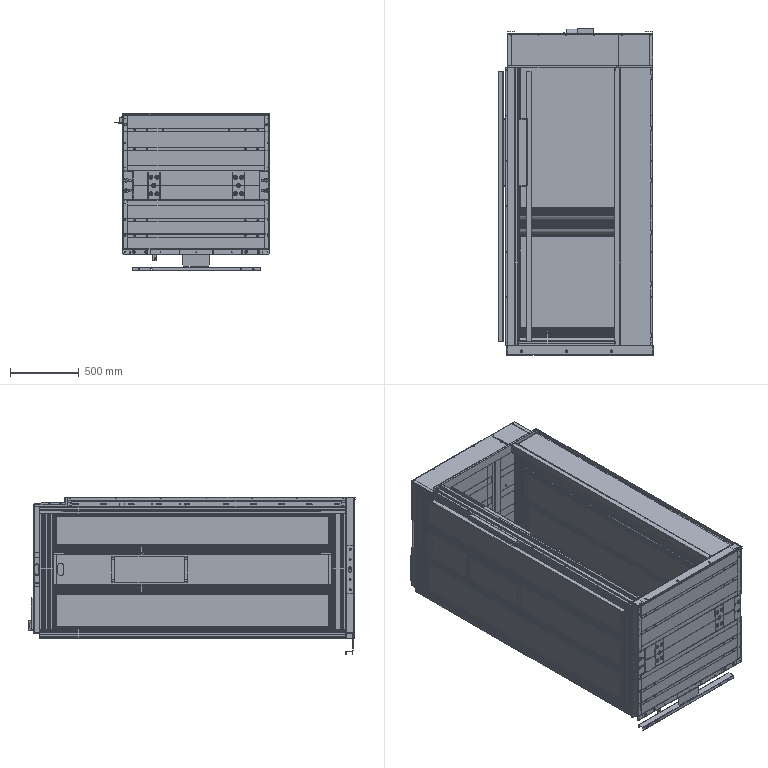Part | 312 solids | 11786 faces | volume 193712455 mm3 | plane 7633 | cylinder 3967 | cone 186 | commonest cylinder face diameters 10 x333 0.4 x325 6 x271 1.1 x240 11 x235 3.6 x228